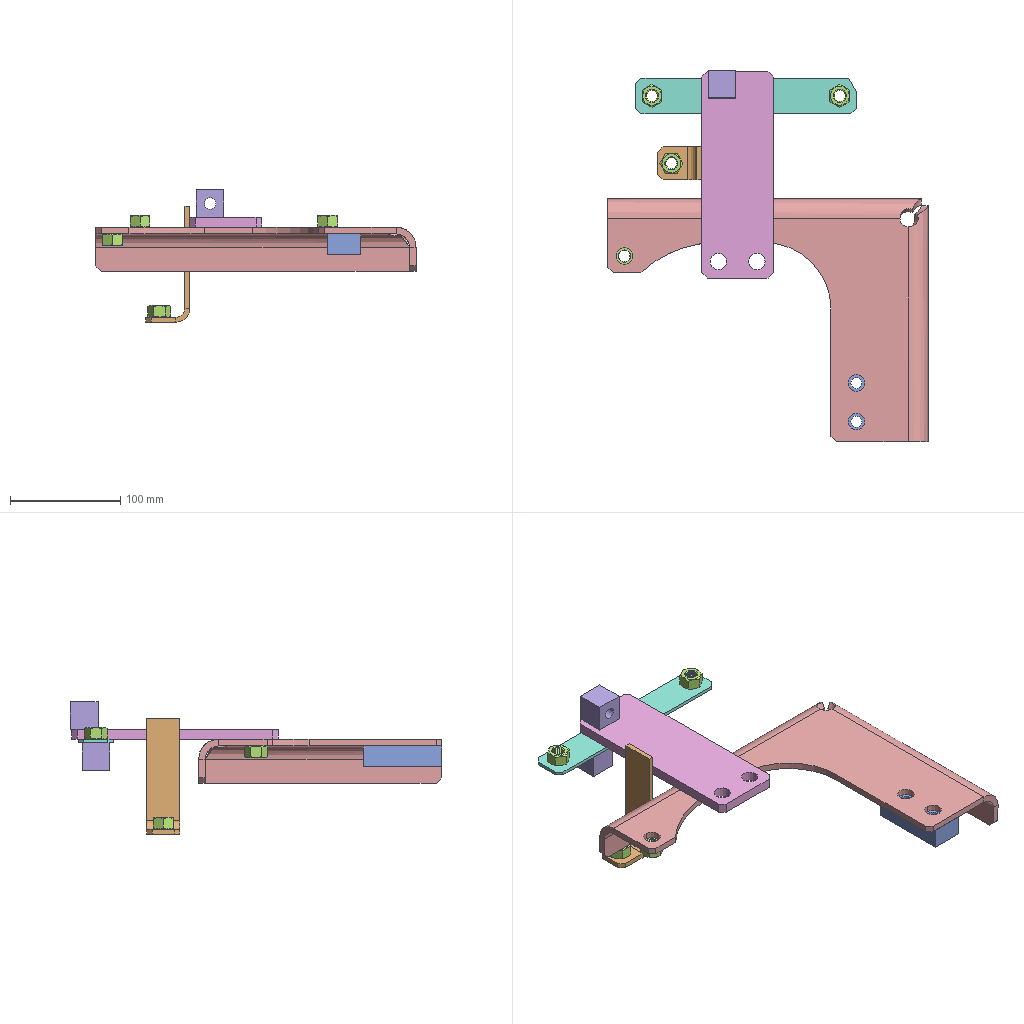Assembly | SolidWorks | 9 different items | 13 placed | box 290 x 336 x 120 mm
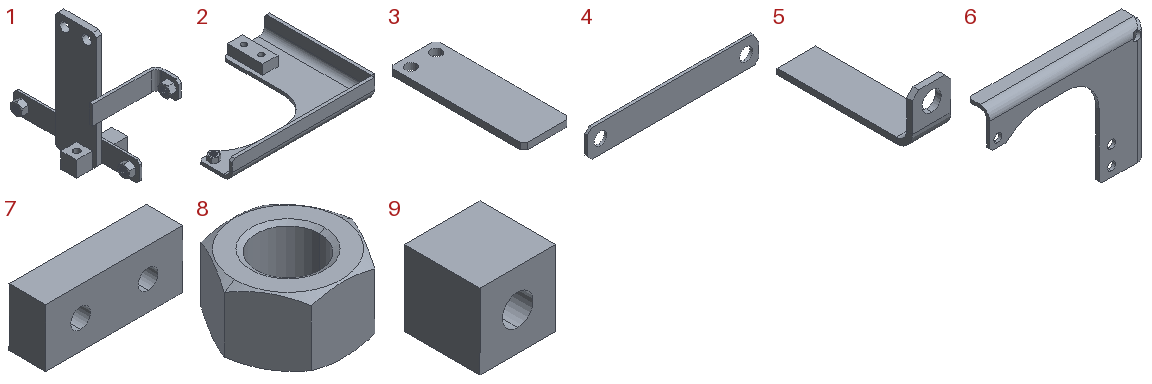Parts list (item | name | quantity | parent item | size | volume | features):
1 | (subassembly) | x1 | - | 120 x 200 x 188 mm | 175501 mm3 | -
2 | (subassembly) | x1 | - | 290 x 220 x 40 mm | 293672 mm3 | -
3 | - | x1 | in 1 | 65 x 187 x 9 mm | 105764 mm3 | features FlatPattern 1, SMBaseFlange 1, SheetMetal 1
4 | - | x1 | in 1 | 200 x 3.2 x 32 mm | 19095 mm3 | features FlatPattern 1, SMBaseFlange 1, SheetMetal 1
5 | - | x1 | in 1 | 30 x 105 x 40 mm | 17466 mm3 | features Chamfer 1, FlatPattern 1, ICE 1, SMBaseFlange 1, SheetMetal 1
6 | - | x1 | in 2 | 290 x 40 x 220 mm | 254298 mm3 | features Chamfer 1, EdgeFlange 1, FlatPattern 1, Fold 1, ICE 1, SMBaseFlange 1, SheetMetal 1, UnFold 1
7 | - | x1 | in 2 | 71 x 19 x 30 mm | 37365 mm3 | features FlatPattern 1, HoleWzd 1, SMBaseFlange 1, SheetMetal 1
8 | - | x4 | in 1, 2 | 27.713 x 24 x 14.8 mm | 5071 mm3 | features RevCut 2, Chamfer 1, Extrusion 1, LPattern 1
9 | - | x2 | in 1 | 25 x 25 x 25 mm | 13582 mm3 | features Extrusion 1, HoleWzd 1
Mates (type | each side: item.copy, entity, surface, feature):
In the top assembly
Coincident | 6.1 face plane Base-Flange1 | 3.1 face plane Base-Flange1
DistanceDim | 6.1 face plane Base-Flange1 | 3.1 face plane Base-Flange1 | 2 times
In subassembly 2
Coincident | 6.2 face plane Base-Flange1 | 7.1 face plane Base-Flange1
Concentric | 6.2 face cylinder Base-Flange1 | 7.1 face cylinder M12 Tapped Hole1 | 2 times
Concentric | 6.2 face cylinder Base-Flange1 | 8.1 face cone EndChamfer
Coincident | 6.2 face plane Base-Flange1 | 8.1 face plane BaseNut
Parallel | 6.2 face plane Base-Flange1 | 8.1 face plane BaseNut
In subassembly 1
Coincident | 3.2 face plane Base-Flange1 | 1.1 plane | 3 times
Coincident | 3.2 face plane Base-Flange1 | 4.1 face plane Base-Flange1
DistanceDim | 3.2 face plane Base-Flange1 | 4.1 face plane Base-Flange1 | 2 times
Coincident | 3.2 face plane Base-Flange1 | 5.1 face plane Base-Flange1
DistanceDim | 3.2 face plane Base-Flange1 | 5.1 face plane Base-Flange1
DistanceDim | 5.1 face plane Base-Flange1 | 3.2 face plane Base-Flange1
Concentric | 5.1 face cylinder Cut-Extrude1 | 8.1 face cone EndChamfer
Coincident | 5.1 face plane Base-Flange1 | 8.1 face plane BaseNut
Parallel | 5.1 face plane Base-Flange1 | 8.1 face plane BaseNut
Concentric | 4.1 face cylinder Base-Flange1 | 8.2 face cone EndChamfer
Coincident | 4.1 face plane Base-Flange1 | 8.2 face plane BaseNut
Concentric | 4.1 face cylinder Base-Flange1 | 8.3 face cone EndChamfer
Coincident | 4.1 face plane Base-Flange1 | 8.3 face plane BaseNut
Parallel | 4.1 face plane Base-Flange1 | 8.3 face plane BaseNut
Parallel | 4.1 face plane Base-Flange1 | 8.2 face plane BaseNut
Coincident | 3.2 face plane Base-Flange1 | 9.1 face plane Boss-Extrude1
DistanceDim | 3.2 face plane Base-Flange1 | 9.1 face plane Boss-Extrude1
DistanceDim | 9.1 face plane Boss-Extrude1 | 3.2 face plane Base-Flange1
Coincident | 4.1 face plane Base-Flange1 | 9.2 face plane Boss-Extrude1
DistanceDim | 9.2 face plane Boss-Extrude1 | 4.1 face plane Base-Flange1 | 2 times